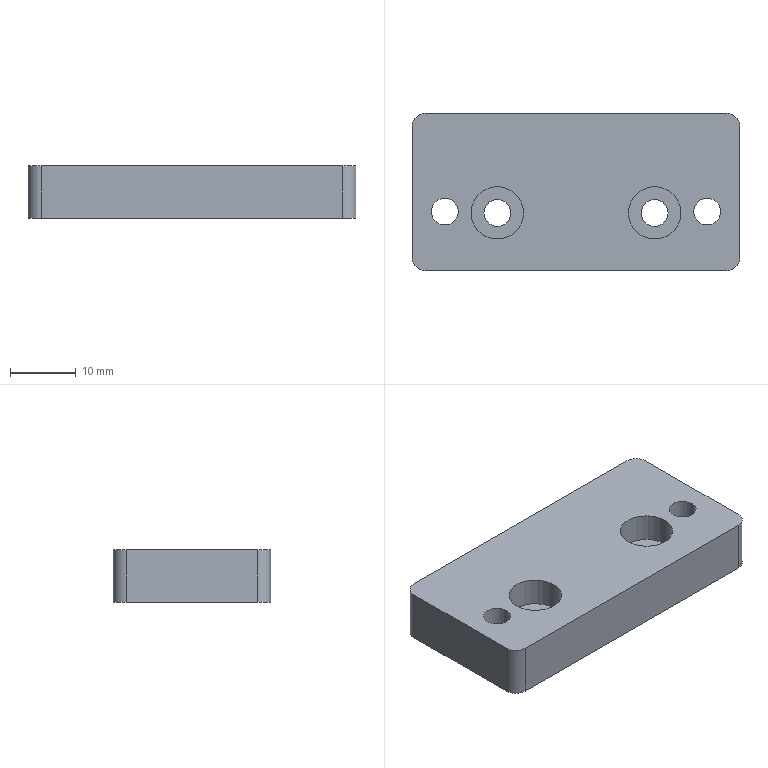Part | STEP file | 1 solid | 30 faces | box 50 x 24 x 8 mm | volume 8483 mm3 | cylinder 20 | plane 10 | commonest cylinder face diameters 4.1 x8 8 x8 4 x4